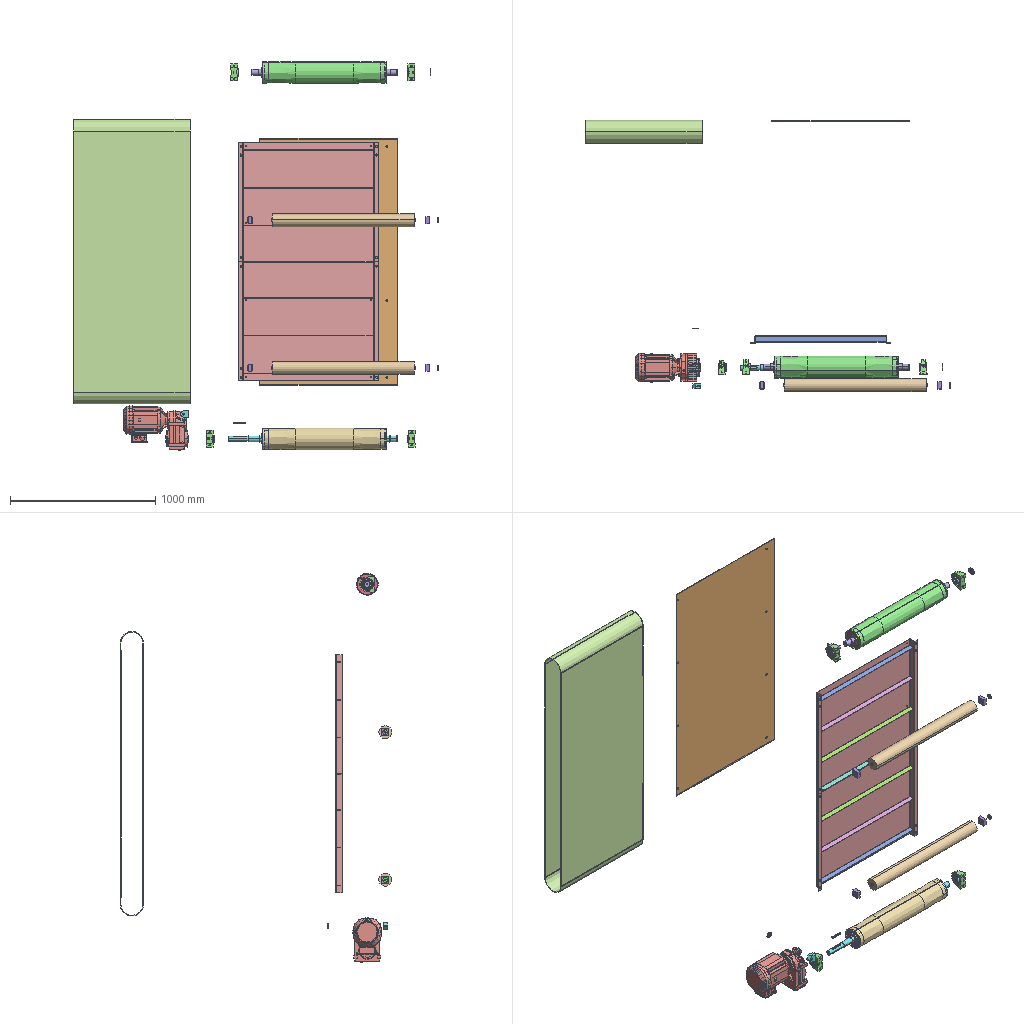Assembly | SolidWorks | 34 different items | 93 placed | box 2508 x 1869 x 2679 mm
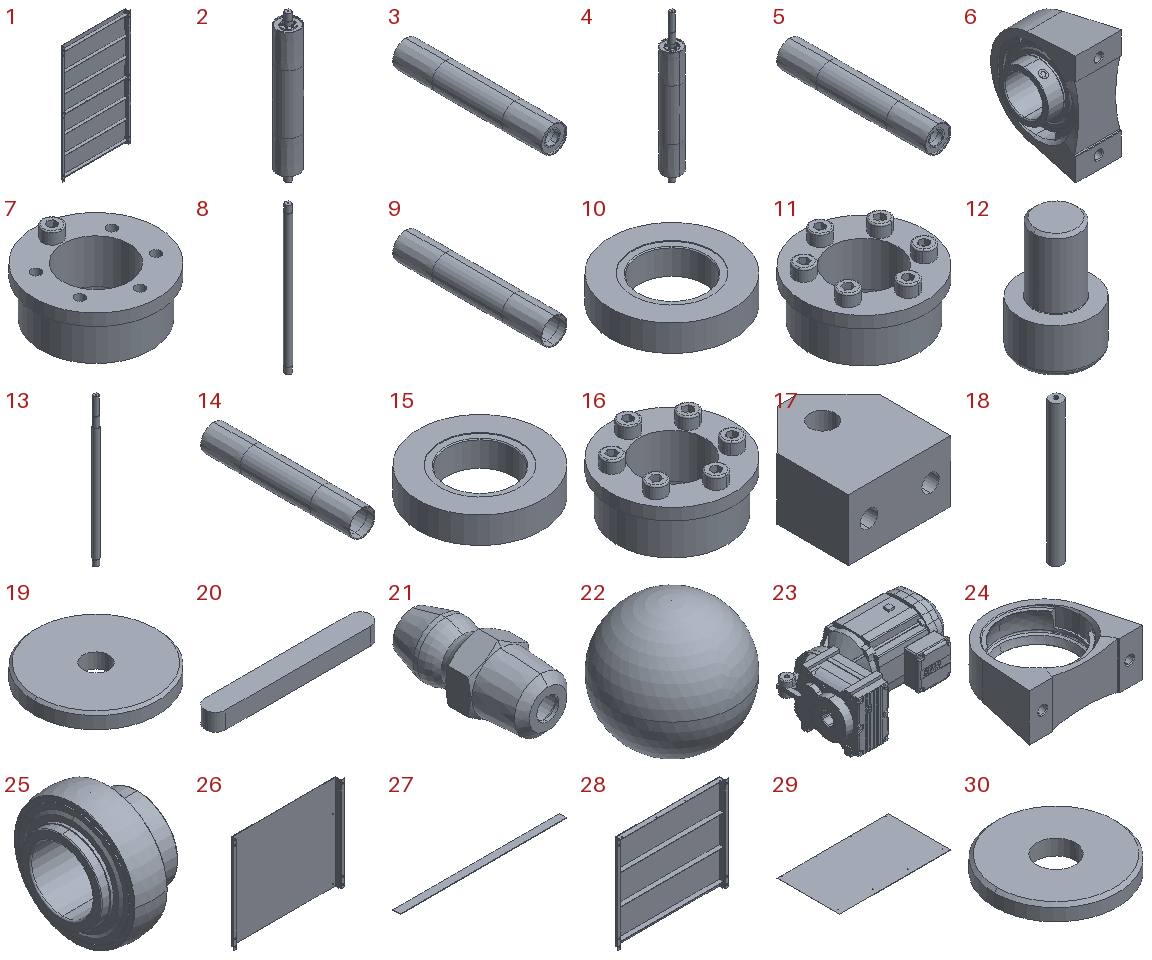Parts list (item | name | quantity | parent item | size | volume | features):
1 | (subassembly) | x1 | - | 966 x 49 x 1640 mm | 6033674 mm3 | -
2 | (subassembly) | x1 | - | 150 x 150 x 1000 mm | 4622991 mm3 | -
3 | (subassembly) | x1 | - | 150 x 850 x 150 mm | 2873344 mm3 | features CompositeCurve 1
4 | (subassembly) | x1 | - | 150 x 150 x 1164 mm | 4781724 mm3 | -
5 | (subassembly) | x1 | - | 150 x 850 x 150 mm | 2873344 mm3 | features CompositeCurve 1
6 | (subassembly) | x4 | - | 54.2 x 99.5 x 116 mm | 238487 mm3 | features AEMSimFeature 1
7 | - | x1 | - | 84 x 84 x 41 mm | 89359 mm3 | features BaseBody 3, ICE 1
8 | - | x1 | in 2 | 45 x 45 x 1000 mm | 1555641 mm3 | features HoleWzd 2, ICE 2, Chamfer 1, Extrusion 1, Fillet 1
9 | - | x1 | in 2 | 150 x 850 x 150 mm | 2218913 mm3 | features ICE 3, Chamfer 1, Revolution 1
10 | - | x2 | in 2 | 140 x 140 x 30 mm | 327215 mm3 | features Chamfer 1, Extrusion 1, ICE 1
11 | - | x2 | in 2 | 84 x 84 x 41 mm | 97003 mm3 | features BaseBody 8
12 | - | x1 | - | 13 x 13 x 20 mm | 1529 mm3 | features Fillet 2, ICE 2, Chamfer 1, Extrusion 1
13 | - | x1 | in 4 | 45 x 45 x 1164 mm | 1714375 mm3 | features ICE 4, Chamfer 2, HoleWzd 2, Extrusion 1, Fillet 1
14 | - | x1 | in 4 | 150 x 850 x 150 mm | 2218913 mm3 | features ICE 3, Chamfer 1, Revolution 1
15 | - | x2 | in 4 | 140 x 140 x 30 mm | 327215 mm3 | features Chamfer 1, Extrusion 1, ICE 1
16 | - | x2 | in 4 | 84 x 84 x 41 mm | 97003 mm3 | features BaseBody 8
17 | - | x1 | - | 50 x 55 x 30 mm | 63941 mm3 | features Chamfer 1, Extrusion 1, HoleWzd 1, ICE 1
18 | - | x2 | - | 89 x 89 x 992 mm | 5903477 mm3 | features ICE 3, HoleWzd 2, Extrusion 1
19 | - | x1 | - | 50 x 50 x 6 mm | 11184 mm3 | features Chamfer 1, Extrusion 1
20 | - | x1 | - | 80 x 10 x 8.3 mm | 6462 mm3 | features Extrusion 1
21 | - | x4 | in 6 | 7.001 x 16.4 x 8.083 mm | 360.824 mm3 | features BaseBody 1
22 | - | x36 | in 6 | 12.303 x 12.303 x 12.303 mm | 975.061 mm3 | features BaseBody 1
23 | - | x1 | - | 447.5 x 307.56 x 199 mm | 13556932 mm3 | features MBimport 1
24 | - | x4 | in 6 | 116 x 99.5 x 48 mm | 160162 mm3 | features BaseBody 1
25 | - | x4 | in 6 | 49.2 x 80 x 80 mm | 69188 mm3 | features BaseBody 1
26 | - | x1 | - | 966 x 49 x 820 mm | 2585319 mm3 | features ICE 2, Extrusion 1
27 | - | x1 | - | 900 x 40 x 3 mm | 107995 mm3 | features Extrusion 1, Fillet 1
28 | - | x2 | in 1 | 966 x 49 x 820 mm | 3016837 mm3 | features BaseBody 5, ICE 1
29 | - | x1 | - | 1700 x 950 x 3 mm | 4835265 mm3 | features ICE 2, Extrusion 1
30 | - | x1 | - | 40 x 40 x 5 mm | 5608 mm3 | features Chamfer 1, Extrusion 1
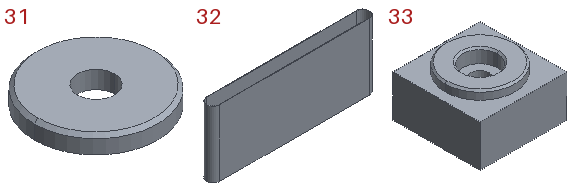31 | - | x4 | - | 35 x 35 x 5 mm | 4324 mm3 | features Chamfer 1, Extrusion 1
32 | - | x1 | - | 1960 x 160 x 800 mm | 16347787 mm3 | features ExtruThin 1
33 | - | x4 | - | 50 x 50 x 29 mm | 61857 mm3 | features ICE 3, Chamfer 2, Extrusion 1
34 | - | x1 | - | - | - | -
Mates (type | each side: item.copy, entity, surface, feature):
In the top assembly
Coincident | assembly face | 29.1 face plane Boss-Extrude 1
Concentric | assembly edge | 29.1 edge | 2 times
Parallel | 29.1 face plane Boss-Extrude 1 | 10.1 face plane Boss-Extrude 1
Parallel | assembly face | 13.1 face plane Boss-Extrude 3
Coincident | 10.2 face plane Boss-Extrude 1 | 15.1 face plane Boss-Extrude 1
Concentric | 8.1 face cylinder Boss-Extrude 3 | 25.1 face cylinder
Coincident | 8.1 face plane Boss-Extrude 1 | 25.1 face plane
Concentric | 8.1 face cylinder Boss-Extrude 2 | 25.2 face cylinder
Coincident | 8.1 face plane Boss-Extrude 1 | 25.2 face plane
Parallel | 29.1 face plane Boss-Extrude 1 | 24.1 face plane
Coincident | 24.2 face plane | 24.1 face plane
Concentric | 13.1 face cylinder Boss-Extrude 4 | 25.3 face cylinder
Coincident | 13.1 face plane Boss-Extrude 1 | 25.3 face plane
Concentric | 13.1 face cylinder Boss-Extrude 4 | 25.4 face cylinder
Coincident | 13.1 face plane Boss-Extrude 1 | 25.4 face plane
Coincident | 24.3 face plane | 24.4 face plane
Coincident | 24.2 face plane | 24.3 face plane
DistanceDim | 9.1 face cylinder Revolve 1 | 14.1 face cylinder Revolve 1
Width | 10.2 face plane Boss-Extrude 1 | 10.1 face plane Boss-Extrude 1 | assembly face | assembly face
Width | 24.2 face plane | 24.3 face plane | assembly face | assembly face
Coincident | 25.1 face plane | 19.1 face plane Boss-Extrude 1
Concentric | 25.1 face cylinder | 19.1 face cylinder Boss-Extrude 1
Coincident | 13.1 face plane Cut-Extrude 1 | 20.1 face plane Boss-Extrude 1
Concentric | 13.1 face cylinder Cut-Extrude 1 | 20.1 face cylinder Boss-Extrude 1 | 2 times
Coincident | 29.1 face plane Boss-Extrude 1 | 32.1 face plane Extrude-Thin Wall 1
Concentric | 9.1 face cylinder Revolve 1 | 32.1 face cylinder Extrude-Thin Wall 1
Width | 32.1 face plane Extrude-Thin Wall 1 | 32.1 face plane Extrude-Thin Wall 1 | assembly face | assembly face
Parallel | assembly face | 17.1 face plane Boss-Extrude 1
Parallel | 15.2 face plane Boss-Extrude 1 | 18.1 face plane Boss-Extrude 1
Coincident | 18.1 face plane Boss-Extrude 1 | 18.2 face plane Boss-Extrude 1
Width | 18.1 face plane Boss-Extrude 1 | 18.1 face plane Boss-Extrude 1 | assembly face | assembly face
Tangent | 32.1 face plane Extrude-Thin Wall 1 | 18.1 face cylinder Boss-Extrude 1
Tangent | 32.1 face plane Extrude-Thin Wall 1 | 18.2 face cylinder Boss-Extrude 1
DistanceDim | 18.1 face cylinder Boss-Extrude 1 | 18.2 face cylinder Boss-Extrude 1
Coincident | 18.1 face plane Boss-Extrude 2 | 33.1 face plane Boss-Extrude 1
Concentric | 18.1 face cylinder Boss-Extrude 1 | 33.1 face cylinder Cut-Extrude 2
Coincident | 18.2 face plane Boss-Extrude 3 | 33.2 face plane Boss-Extrude 1
Concentric | 18.2 face cylinder Boss-Extrude 1 | 33.2 face cylinder Cut-Extrude 2
Coincident | 33.2 face plane Boss-Extrude 1 | 33.1 face plane Boss-Extrude 1
Parallel | 32.1 face plane Extrude-Thin Wall 1 | 33.1 face plane Boss-Extrude 1
Coincident | 18.1 face plane Boss-Extrude 3 | 33.3 face plane Boss-Extrude 1
Concentric | 18.1 face cylinder Boss-Extrude 1 | 33.3 face cylinder Cut-Extrude 2
Concentric | 18.2 face cylinder Boss-Extrude 1 | 33.4 face cylinder Cut-Extrude 2
Coincident | 18.2 face plane Boss-Extrude 2 | 33.4 face plane Boss-Extrude 1
Coincident | 33.3 face plane Boss-Extrude 1 | 33.4 face plane Boss-Extrude 1
Parallel | 32.1 face plane Extrude-Thin Wall 1 | 33.3 face plane Boss-Extrude 1
Width | 33.2 face plane Boss-Extrude 1 | 33.1 face plane Boss-Extrude 1 | assembly face | assembly face
Coincident | 33.1 face plane Boss-Extrude 1 | 31.1 face plane Boss-Extrude 1
Concentric | 18.1 face cylinder Boss-Extrude 1 | 31.1 face cylinder Boss-Extrude 1
Coincident | 33.3 face plane Boss-Extrude 1 | 31.2 face plane Boss-Extrude 1
Concentric | 18.1 face cylinder Boss-Extrude 1 | 31.2 face cylinder Boss-Extrude 1
Coincident | 33.2 face plane Boss-Extrude 1 | 31.3 face plane Boss-Extrude 1
Concentric | 18.2 face cylinder Boss-Extrude 1 | 31.3 face cylinder Boss-Extrude 1
Coincident | 33.4 face plane Boss-Extrude 1 | 31.4 face plane Boss-Extrude 1
Concentric | 18.2 face cylinder Boss-Extrude 1 | 31.4 face cylinder Boss-Extrude 1
In subassembly 2
Concentric | 8.2 face cylinder Boss-Extrude 1 | 9.2 face cylinder Cut-Extrude 3
Concentric | 9.2 face cone Revolve 1 | 11.1 face cylinder
Concentric | 9.2 face cone Revolve 1 | 10.3 face cylinder Boss-Extrude 1
Coincident | 9.2 face plane Cut-Extrude 2 | 10.3 face plane Boss-Extrude 1
Coincident | 10.3 face plane Cut-Extrude 1 | 11.1 face plane
Concentric | 9.2 face cylinder Cut-Extrude 1 | 10.4 face cylinder Boss-Extrude 1
Concentric | 10.4 face cylinder Boss-Extrude 1 | 11.2 face cylinder
Coincident | 9.2 face plane Cut-Extrude 1 | 10.4 face plane Boss-Extrude 1
Coincident | 10.4 face plane Cut-Extrude 1 | 11.2 face plane
DistanceDim | 8.2 face plane Boss-Extrude 3 | 9.2 face plane Revolve 1
In subassembly 4
Concentric | 14.2 face cylinder Cut-Extrude 1 | 15.3 face cylinder Boss-Extrude 1
Coincident | 14.2 face plane Cut-Extrude 1 | 15.3 face plane Boss-Extrude 1
Concentric | 13.2 face cylinder Boss-Extrude 1 | 15.3 face cylinder Boss-Extrude 1
Concentric | 15.3 face cylinder Boss-Extrude 1 | 16.1 face cylinder
Coincident | 15.3 face plane Cut-Extrude 1 | 16.1 face plane
Concentric | 14.2 face cylinder Cut-Extrude 2 | 15.4 face cylinder Boss-Extrude 1
Concentric | 15.4 face cylinder Boss-Extrude 1 | 16.2 face cylinder
Coincident | 15.4 face plane Cut-Extrude 1 | 16.2 face plane
Coincident | 14.2 face plane Cut-Extrude 2 | 15.4 face plane Boss-Extrude 1
DistanceDim | 14.2 face plane Revolve 1 | 13.2 face plane Boss-Extrude 3
In subassembly 1
Coincident | 28.1 face plane | 28.2 face plane | 3 times